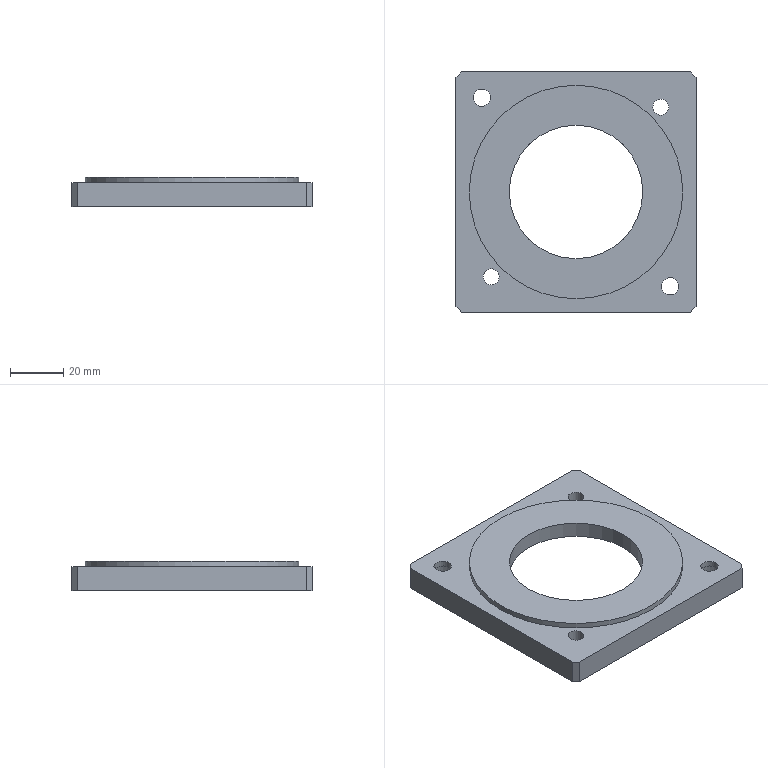NC program | NX | posted with a generic post | part box 90 x 90 x 11 mm
Lines 1 to 1755 of 1862, first 1544 of 1739 lines:
N10 G17 G21 G94 G90
(FLOOR_WALL , TOOL : D50)
N12 T15 M6
N14 G54
N16 G17 G0 G90 X-76.5 Y48.497 S6500 M3
N18 G43 Z30. H15
N20 Z3.
N22 G94 G1 Z0. F1250.
N24 X-73.5
N26 X73.5
N28 Y9.999
N30 X-73.5
N32 Y-28.5
N34 X73.5
N36 X76.5
N38 Z3.
N40 G0 Z30.
N42 M5
(ADAPTIVE_MILLING , TOOL : D10)
N44 T10 M6
N46 G54
N48 G17 G0 G90 X-56.209 Y-0.062 S9500 M3
N50 G43 Z30. H10
N52 Z-8.
N54 G94 G1 Z-11. F1000.
N56 X-55.429 Y-0.341 F3000.
N58 X-54.64 Y-0.597
N60 G3 X-53.562 Y-0.062 R1.017
N62 X-52.789 Y3.126 R8.525
N64 X-52.52 Y12.494 R110.617
N66 G1 X-52.514 Y14.619
N68 X-52.511 Y17.994
N70 X-52.51 Y26.869
N72 X-52.509 Y45.369
N74 Y45.494
N76 X-52.507 Y45.619
N78 G2 X-50.114 Y49.825 R5.686
N80 X-44.574 Y51.965 R12.187
N82 X-36.471 Y52.453 R57.565
N84 G1 X-35.471 Y52.463
N86 X-34.346 Y52.471
N88 X-32.721 Y52.479
N90 X-30.596 Y52.484
N92 X-27.096 Y52.487
N94 X-17.221 Y52.488
N96 X28.779
N98 X29.529 Y52.492
N100 X30.654 Y52.493
N102 X31.529
N104 X32.279 Y52.496
N106 X33.404 Y52.495
N108 G2 X46.028 Y52.466 R533.587
N110 X50.208 Y49.565 R6.086
N112 X52.064 Y43.911 R13.666
N114 X52.471 Y34.426 R81.29
N116 G1 X52.478 Y32.926
N118 X52.483 Y30.801
N120 X52.487 Y27.426
N122 X52.488 Y19.051
N124 X52.489 Y-29.449
N126 X52.495 Y-30.949
N128 X52.494 Y-32.449
N130 X52.496 Y-33.074
N132 Y-34.199
N134 X52.495 Y-34.824
N136 X52.498 Y-35.699
N138 X52.497 Y-36.699
N140 X52.499 Y-37.699
N142 X52.497 Y-38.949
N144 X52.498 Y-39.574
N146 X52.497 Y-40.949
N148 Y-41.449
N150 X52.499 Y-42.449
N152 X52.497 Y-43.574
N154 X52.499 Y-44.324
N156 X52.498 Y-45.324
N158 X52.497 Y-45.574
N160 X52.494 Y-45.699
N162 X52.487 Y-45.824
N164 X52.475 Y-45.949
N166 G2 X49.63 Y-50.163 R6.032
N168 X43.988 Y-52.053 R13.529
N170 X34.878 Y-52.467 R76.098
N172 G1 X33.503 Y-52.475
N174 X31.628 Y-52.481
N176 X28.878 Y-52.485
N178 X23.503 Y-52.487
N180 X-45.497 Y-52.488
N182 X-45.622 Y-52.486
N184 G2 X-49.826 Y-50.086 R5.702
N186 X-51.945 Y-44.67 R12.092
N188 X-52.451 Y-36.568 R56.305
N190 G1 X-52.462 Y-35.568
N192 X-52.47 Y-34.443
N194 X-52.477 Y-33.068
N196 X-52.483 Y-31.068
N198 X-52.486 Y-27.943
N200 X-52.488 Y-21.068
N202 Y-3.818
N204 X-52.487 Y-3.693
N206 X-52.485 Y-3.568
N208 X-52.478 Y-3.318
N210 X-52.473 Y-3.193
N212 G2 X-51.832 Y3.148 R397.339
N214 G3 X-51.526 Y17.267 R210.01
N216 G1 X-51.522 Y20.767
N218 X-51.52 Y28.392
N220 Y42.392
N222 X-51.518 Y42.517
N224 X-51.516 Y42.642
N226 X-51.504 Y42.891
N228 G2 X-47.72 Y48.895 R7.721
N230 X-41.356 Y50.984 R15.76
N232 X-31.249 Y51.454 R84.679
N234 G1 X-29.874 Y51.462
N236 X-28.124 Y51.469
N238 X-25.749 Y51.473
N240 X-21.624 Y51.476
N242 X-7.499 Y51.477
N244 X25.751
N246 G2 X43.125 Y51.466 R849.618
N248 X48.889 Y47.718 R7.741
N250 X50.999 Y41.231 R15.861
N252 X51.45 Y31.748 R82.109
N254 G1 X51.458 Y30.623
N256 X51.466 Y28.998
N258 X51.472 Y26.998
N260 X51.475 Y23.998
N262 X51.477 Y17.748
N264 X51.478 Y-26.502
N266 G2 X51.464 Y-43.126 R752.147
N268 X47.716 Y-48.889 R7.737
N270 X41.229 Y-50.999 R15.895
N272 X31.371 Y-51.452 R84.867
N274 G1 X29.996 Y-51.461
N276 X28.246 Y-51.468
N278 X25.746 Y-51.473
N280 X21.621 Y-51.476
N282 X7.496 Y-51.477
N284 X-42.379
N286 G2 X-48.754 Y-47.906 R7.59
N288 X-50.909 Y-41.829 R14.89
N290 X-51.435 Y-33.102 R65.156
N292 G1 X-51.446 Y-32.102
N294 X-51.456 Y-30.852
N296 X-51.464 Y-29.352
N298 X-51.47 Y-27.352
N300 X-51.475 Y-24.477
N302 X-51.477 Y-18.977
N304 G2 X-51.429 Y-4.228 R621.113
N306 G3 X-50.742 Y5.247 R678.078
N308 X-50.532 Y25.994 R547.933
N310 G2 X-50.492 Y40.743 R710.406
N312 X-50.15 Y42.711 R15.101
N314 X-48.663 Y46.614 R5.592
N316 G1 X-48.617 Y46.666
N318 X-46.666 Y48.617
N320 X-46.614 Y48.663
N322 G2 X-43.034 Y50.145 R5.569
N324 G3 X-33.719 Y50.406 R849.439
N326 G2 X-16.22 Y50.466 R903.691
N328 G1 X22.78
N330 X23.905 Y50.473
N332 X24.905 Y50.474
N334 X25.78 Y50.475
N336 X26.655 Y50.479
N338 X27.405 Y50.481
N340 G2 X40.779 Y50.46 R547.914
N342 X42.624 Y50.15 R18.518
N344 X45.63 Y49.418 R5.935
N346 G1 X46.614 Y48.663
N348 X46.666 Y48.617
N350 X48.617 Y46.666
N352 X48.663 Y46.614
N354 G2 X50.145 Y43.034 R5.569
N356 G3 X50.412 Y33.344 R935.35
N358 G1 X50.426 Y32.095
N360 X50.438 Y30.72
N362 X50.447 Y29.095
N364 X50.456 Y27.095
N366 X50.461 Y24.595
N368 X50.465 Y20.845
N370 X50.467 Y12.72
N372 Y-23.53
N374 X50.473 Y-24.655
N376 X50.474 Y-25.655
N378 X50.475 Y-26.655
N380 X50.481 Y-27.655
N382 G2 X50.459 Y-40.779 R542.291
N384 X50.15 Y-42.62 R17.941
N386 X49.418 Y-45.63 R5.937
N388 G1 X48.663 Y-46.614
N390 X48.617 Y-46.666
N392 X46.666 Y-48.617
N394 X46.614 Y-48.663
N396 G2 X43.034 Y-50.145 R5.569
N398 G3 X33.469 Y-50.409 R920.282
N400 G2 X14.095 Y-50.466 R996.301
N402 G1 X-39.78
N404 X-40.03 Y-50.464
N406 X-40.28 Y-50.458
N408 X-40.405 Y-50.454
N410 X-40.655 Y-50.441
N412 G2 X-42.517 Y-50.15 R16.061
N414 X-45.63 Y-49.418 R5.996
N416 G1 X-46.614 Y-48.663
N418 X-46.666 Y-48.617
N420 X-48.617 Y-46.666
N422 X-48.663 Y-46.614
N424 G2 X-50.145 Y-43.034 R5.569
N426 G3 X-50.402 Y-33.844 R791.933
N428 G1 X-50.417 Y-32.719
N430 X-50.43 Y-31.47
N432 X-50.44 Y-30.22
N434 X-50.449 Y-28.595
N436 X-50.457 Y-26.47
N438 X-50.462 Y-23.97
N440 X-50.465 Y-19.845
N442 G2 X-50.416 Y-5.345 R679.932
N444 G1 X-50.395 Y-4.846
N446 X-50.371 Y-4.346
N448 X-50.344 Y-3.847
N450 X-50.313 Y-3.348
N452 X-50.271 Y-2.724
N454 X-50.191 Y-1.602
N456 X-50.15 Y-1.046
N458 Y42.829
N460 G2 X-49.418 Y45.63 R5.894
N462 G1 X-48.617 Y46.666
N464 X-46.614 Y48.663
N466 G2 X-44.264 Y49.984 R5.901
N468 X-41.965 Y50.15 R11.351
N470 G1 X42.66
N472 G2 X45.63 Y49.418 R5.92
N474 G1 X46.666 Y48.617
N476 X48.663 Y46.614
N478 G2 X49.984 Y44.264 R5.901
N480 X50.15 Y41.84 R11.646
N482 G1 Y-42.66
N484 G2 X49.418 Y-45.63 R5.92
N486 G1 X48.617 Y-46.666
N488 X46.614 Y-48.663
N490 G2 X44.264 Y-49.984 R5.901
N492 X41.84 Y-50.15 R11.646
N494 G1 X-42.535
N496 G2 X-45.63 Y-49.418 R5.985
N498 G1 X-46.666 Y-48.617
N500 X-48.663 Y-46.614
N502 G2 X-49.984 Y-44.264 R5.901
N504 X-50.15 Y-41.84 R11.646
N506 G1 Y-0.965
N508 G3 X-50.998 Y0.032 R1.016
N510 G1 X-52.551 Y0.284
N512 Z-8.
N514 G0 Z30.
N516 X-52.802 Y0.345
N518 Z1.151
N520 G1 Z-1.849 F1000.
N522 X-52.021 Y0.066 F3000.
N524 X-51.233 Y-0.191
N526 G3 X-50.155 Y0.345 R1.017
N528 X-49.394 Y3.409 R8.28
N530 X-49.111 Y13.276 R111.643
N532 G1 X-49.107 Y15.526
N534 X-49.104 Y19.401
N536 X-49.103 Y33.026
N538 Y39.901
N540 X-49.102 Y40.026
N542 X-49.1 Y40.151
N544 G2 X-46.974 Y45.635 R8.713
N546 X-41.836 Y48.307 R10.099
N548 X-34.132 Y49.017 R38.987
N550 X-14.882 Y49.081 R957.171
N552 G1 X39.993
N554 X40.118 Y49.08
N556 X40.242 Y49.078
N558 X40.367 Y49.074
N560 X40.492 Y49.067
N562 X40.617 Y49.058
N564 G2 X45.787 Y46.806 R8.398
N566 X48.354 Y41.609 R10.436
N568 X49.012 Y34.4 R39.109
N570 X49.08 Y21.15 R718.348
N572 G1 X49.081 Y-11.975
N574 Y-40.1
N576 X49.079 Y-40.225
N578 X49.075 Y-40.35
N580 X49.069 Y-40.474
N582 G2 X46.831 Y-45.783 R8.537
N584 X41.753 Y-48.315 R10.23
N586 X34.547 Y-48.991 R37.77
N588 X18.922 Y-49.065 R791.179
N590 G1 X-40.078 Y-49.08
N592 X-40.203 Y-49.079
N594 X-40.328 Y-49.075
N596 X-40.453 Y-49.07
N598 X-40.578 Y-49.062
N600 G2 X-45.769 Y-46.852 R8.524
N602 X-48.352 Y-41.664 R10.293
N604 X-49.009 Y-34.581 R38.201
N606 X-49.08 Y-21.331 R714.275
N608 G1 X-49.081 Y-3.456
N610 X-49.08 Y-3.331
N612 X-49.075 Y-3.081
N614 X-49.072 Y-2.956
N616 X-49.061 Y-2.707
N618 G2 X-48.441 Y3.386 R677.891
N620 G3 X-48.123 Y16.004 R179.253
N622 G1 X-48.118 Y18.629
N624 X-48.115 Y22.879
N626 X-48.113 Y36.129
N628 Y37.004
N630 X-48.109 Y37.504
N632 X-48.104 Y37.754
N634 G2 X-46.562 Y43.071 R9.233
N636 X-41.076 Y46.799 R10.478
N638 X-33.555 Y47.912 R29.339
N640 X-19.557 Y48.068 R385.711
N642 G1 X-12.557 Y48.07
N644 X37.443
N646 X37.568 Y48.069
N648 X37.693 Y48.067
N650 X37.943 Y48.061
N652 X38.068 Y48.056
N654 G2 X43.989 Y45.782 R8.629
N656 X47.123 Y39.907 R11.849
N658 X47.965 Y32.217 R38.476
N660 X48.069 Y17.718 R712.107
N662 G1 X48.07 Y4.593
N664 Y-37.407
N666 X48.068 Y-37.657
N668 X48.066 Y-37.782
N670 X48.059 Y-38.032
N672 X48.054 Y-38.157
N674 G2 X43.105 Y-45.955 R8.584
N676 X36.615 Y-47.671 R18.662
N678 X25.251 Y-48.041 R122.678
N680 G1 X23.251 Y-48.047
N682 X20.376 Y-48.052
N684 X14.626 Y-48.055
N686 X-37.374 Y-48.069
N688 X-37.499 Y-48.068
N690 X-37.624 Y-48.067
N692 G2 X-42.76 Y-46.758 R9.416
N694 X-46.725 Y-41.303 R10.165
N696 X-47.896 Y-33.919 R27.464
N698 X-48.069 Y-17.546 R401.563
N700 X-48.018 Y-3.797 R500.362
N702 G3 X-47.32 Y6.052 R462.364
N704 X-47.126 Y24.55 R515.339
N706 G2 X-47.064 Y36.674 R391.589
N708 X-41.956 Y44.594 R9.378
N710 X-34.907 Y46.603 R19.29
N712 X-24.671 Y47.033 R100.142
N714 G1 X-23.171 Y47.042
N716 X-21.296 Y47.049
N718 X-18.796 Y47.055
N720 X-14.796 Y47.058
N722 X-4.796 Y47.06
N724 X35.204
N726 G2 X40.208 Y46.18 R11.551
N728 X45.158 Y40.773 R10.187
N730 X46.755 Y33.352 R23.648
N732 X47.047 Y21.983 R163.986
N734 G1 X47.053 Y19.733
N736 X47.057 Y16.483
N738 X47.059 Y9.858
N740 X47.06 Y-35.142
N742 X47.058 Y-35.392
N744 X47.053 Y-35.767
N746 G2 X45.021 Y-42.057 R9.669
N748 X38.943 Y-45.803 R12.014
N750 X30.91 Y-46.885 R34.429
N752 X15.412 Y-47.043 R470.302
N754 G1 X6.162 Y-47.047
N756 X-35.088 Y-47.058
N758 X-35.463 Y-47.055
N760 X-35.713 Y-47.053
N762 X-36.088 Y-47.044
N764 X-36.338 Y-47.035
N766 G2 X-44.679 Y-41.785 R9.402
N768 X-46.613 Y-34.842 R19.415
N770 X-47.035 Y-24.481 R102.047
N772 G1 X-47.043 Y-23.106
N774 X-47.05 Y-21.356
N776 X-47.055 Y-18.856
N778 X-47.058 Y-14.731
N780 X-47.059 Y-7.606
N782 X-47.057 Y-7.106
N784 G2 X-46.533 Y2.504 R187.393
N786 G3 X-46.145 Y19.621 R286.661
N788 G2 X-46.073 Y34.745 R701.821
N790 X-40.394 Y43.541 R10.158
N792 X-33.212 Y45.552 R20.494
N794 X-21.853 Y46.023 R108.266
N796 G1 X-20.353 Y46.032
N798 X-18.353 Y46.039
N800 X-15.603 Y46.044
N802 X-11.103 Y46.048
N804 X2.397 Y46.049
N806 X33.147
N808 G2 X38.42 Y45.231 R13.214
N810 X43.892 Y39.654 R10.673
N812 X45.664 Y32.147 R23.348
N814 X46.034 Y19.906 R147.756
N816 G1 X46.041 Y17.781
N818 X46.045 Y14.781
N820 X46.048 Y9.656
N822 X46.049 Y-16.719
N824 Y-33.219
N826 X46.042 Y-33.844
N828 G2 X44.44 Y-39.918 R10.848
N830 X38.305 Y-44.421 R11.796
N832 X30.447 Y-45.783 R29.546
N834 X17.451 Y-46.026 R247.642
N836 G1 X14.201 Y-46.032
N838 X8.201 Y-46.035
N840 X-33.174 Y-46.046
N842 X-33.674 Y-46.044
N844 X-34.049 Y-46.038
N846 X-34.424 Y-46.026
N848 G2 X-43.575 Y-40.307 R10.166
N850 X-45.595 Y-32.871 R20.985
N852 X-46.027 Y-21.384 R118.173
N854 X-45.989 Y-5.76 R614.756
N856 G3 X-45.275 Y9.097 R676.94
N858 X-45.132 Y30.096 R982.975
N860 G2 X-44.787 Y35.199 R25.006
N862 X-38.871 Y42.528 R10.781
N864 X-31.303 Y44.548 R22.208
N866 X-19.317 Y45.014 R121.813
N868 G1 X-17.567 Y45.023
N870 X-15.567 Y45.029
N872 X-12.692 Y45.034
N874 X-7.817 Y45.037
N876 X-2.695 Y45.038
N878 G2 X2.475 Y45.081 R45.644
N880 G1 X3.975 Y45.068
N882 X5.35 Y45.06
N884 X6.724 Y45.055
N886 X8.099 Y45.054
N888 X9.224 Y45.055
N890 X9.849 Y45.053
N892 X11.224 Y45.052
N894 X12.224 Y45.053
N896 X13.224 Y45.05
N898 X14.724 Y45.053
N900 X15.599 Y45.05
N902 X16.474 Y45.051
N904 X17.724 Y45.048
N906 X18.974 Y45.051
N908 G2 X33.099 Y45.001 R617.655
N910 X42.536 Y38.817 R10.77
N912 X44.568 Y31.124 R22.445
N914 X45.008 Y20.138 R115.245
N916 G1 X45.019 Y18.513
N918 X45.026 Y16.888
N920 X45.032 Y14.388
N922 X45.036 Y10.638
N924 X45.038 Y3.138
N926 Y2.835
N928 G2 X45.08 Y-4.633 R105.576
N930 G1 X45.072 Y-6.008
N932 X45.066 Y-7.758
N934 X45.062 Y-10.383
N936 X45.06 Y-15.508
N938 Y-30.258
N940 X45.055 Y-31.008
N942 G2 X44.463 Y-36.202 R17.067
N944 X38.667 Y-42.596 R10.881
N946 X31.081 Y-44.556 R22.797
N948 X19.594 Y-44.997 R122.648
N950 G1 X17.969 Y-45.006
N952 X15.969 Y-45.014
N954 X13.094 Y-45.019
N956 X8.469 Y-45.024
N958 X3.032 Y-45.026
N960 G2 X-4.1 Y-45.075 R86.171
N962 G1 X-5.1 Y-45.068
N964 X-6.6 Y-45.061
N966 X-8.6 Y-45.056
N968 X-11.725 Y-45.054
N970 X-18.975
N972 X-30.225 Y-45.056
N974 G2 X-35.326 Y-44.702 R23.76
N976 X-42.537 Y-38.82 R10.772
N978 X-44.526 Y-31.5 R21.773
N980 X-45.01 Y-20.141 R108.059
N982 X-44.914 Y-4.893 R343.056
N984 G3 X-44.99 Y-3.781 R5.445
N986 G1 X-45.148 Y0.331
N988 X-44.929 Y4.448
N990 X-44.924 Y4.497
N992 G3 X-44.238 Y13.461 R57.287
N994 G1 X-44.223 Y14.336
N996 X-44.208 Y15.461
N998 X-44.195 Y16.711
N1000 X-44.185 Y18.086
N1002 X-44.175 Y19.961
N1004 X-44.167 Y22.211
N1006 X-44.161 Y25.211
N1008 X-44.15 Y26.711
N1010 X-44.148 Y27.461
N1012 X-44.14 Y28.461
N1014 X-44.129 Y29.46
N1016 X-44.12 Y30.085
N1018 X-44.112 Y30.46
N1020 X-44.105 Y30.71
N1022 G2 X-42.336 Y37.263 R12.523
N1024 X-35.889 Y42.173 R12.658
N1026 X-27.81 Y43.703 R29.71
N1028 X-13.816 Y44.018 R215.208
N1030 G1 X-10.941 Y44.023
N1032 X-9.941 Y44.024
N1034 X-9.816 Y44.03
N1036 X-9.784 Y44.033
N1038 X-8.391 Y44.362
N1040 X-8.344 Y44.371
N1042 X-4.287 Y44.945
N1044 X-4.243 Y44.949
N1046 X-0.903 Y45.14
N1048 X-0.879 Y45.141
N1050 X2.475 Y45.081
N1052 G2 X8.351 Y44.371 R57.662
N1054 G3 X16.967 Y44.075 R92.067
N1056 G2 X31.217 Y44.007 R868.307
N1058 X38.572 Y41.301 R11.514
N1060 X42.609 Y34.519 R14.11
N1062 X43.833 Y25.624 R38.889
N1064 X44.032 Y9.769 R450.651
N1066 G1 X44.51 Y7.566
N1068 X44.519 Y7.518
N1070 X45.018 Y3.439
N1072 X45.021 Y3.39
N1074 X45.04 Y2.765
N1076 G3 X46.648 Y2.002 R1.002
N1078 X47.043 Y2.622 Z-1.812 R1.224
N1080 G1 X47.485 Y3.793 Z-1.749
N1082 X48.195 Y5.699
N1084 X48.222 Y5.947
N1086 X48.17 Y9.319
N1088 X48.068 Y12.689
N1090 X47.931 Y14.933
N1092 X47.748 Y17.172
N1094 X46.55 Y29.756
N1096 G3 X44.724 Y37.824 R32.889
N1098 X41.744 Y42.425 R13.191
N1100 G1 X40.117 Y44.036
N1102 G3 X38.414 Y45.179 R7.647
N1104 X35.662 Y46.344 R26.625
N1106 X33.718 Y46.728 R8.766
N1108 X25.617 Y47.203 R154.579
N1110 G1 X10.913 Y47.633
N1112 X10.71 Y47.614
N1114 X10.512 Y47.562
N1116 X8.706 Y46.839
N1118 X8.048 Y46.577 Z-1.784
N1120 X7.395 Y46.302 Z-1.82
N1122 G3 X7.003 Y45.882 Z-1.849 R1.051
N1124 X7.731 Y44.451 R1.003
N1126 G2 X11.646 Y43.595 R39.336
N1128 G3 X18.997 Y43.113 R47.939
N1130 G2 X29.871 Y42.993 R594.457
N1132 X37.151 Y40.386 R12.045
N1134 X41.392 Y33.732 R14.01
N1136 X42.78 Y24.738 R36.574
N1138 X43.024 Y13.532 R352.44
N1140 X44.036 Y9.75 R25.435
N1142 G3 X45.994 Y9.769 R1.
N1144 G1 X46.149 Y11.763 Z-1.749
N1146 X46.286 Y13.647
N1148 X46.289 Y17.395
N1150 X46.272 Y21.144
N1152 G3 X45.392 Y29.816 R56.113
N1154 G1 X44.709 Y33.501
N1156 G3 X42.554 Y38.63 R15.172
N1158 G1 X42.193 Y39.135
N1160 X41.816 Y39.629
N1162 X40.865 Y40.804
N1164 X39.902 Y41.969
N1166 G3 X34.025 Y45.353 R10.912
N1168 X28.477 Y46.122 R33.819
N1170 G1 X14.46 Y46.851
N1172 X14.236 Y46.834
N1174 X14.02 Y46.774
N1176 X12.236 Y46.022
N1178 X11.611 Y45.764 Z-1.783
N1180 X10.995 Y45.485 Z-1.817
N1182 G3 X10.592 Y44.993 Z-1.849 R1.042
N1184 X11.278 Y43.669 R1.004
N1186 G2 X14.682 Y42.721 R87.973
N1188 G3 X21.648 Y42.143 R39.423
N1190 G2 X29.393 Y41.917 R116.86
N1192 X39.404 Y34.824 R12.046
N1194 X41.51 Y26.503 R25.325
N1196 X41.965 Y16.642 R121.15
N1198 G3 X42.387 Y15.548 R20.046
N1200 G1 X43.027 Y13.522
N1202 G3 X44.814 Y13.269 R1.001
N1204 X44.994 Y13.94 Z-1.814 R1.286
N1206 G1 X45.101 Y15.231 Z-1.749
N1208 X45.277 Y17.419
N1210 X45.266 Y21.434
N1212 G3 X44.718 Y26.744 R35.25
N1214 G1 X43.998 Y30.633
N1216 G3 X42.231 Y35.906 R24.086
N1218 X40.361 Y38.908 R17.781
N1220 G1 X39.408 Y40.143
N1222 X38.419 Y41.351
N1224 G3 X37.476 Y42.151 R4.49
N1226 G1 X35.96 Y43.084
N1228 G3 X32.996 Y44.213 R11.072
N1230 X27.468 Y45.126 R43.094
N1232 G1 X17.02 Y46.133
N1234 G3 X16.512 Y46.048 R1.113
N1236 G1 X14.808 Y45.277
N1238 X14.206 Y45.01 Z-1.782
N1240 X13.614 Y44.72 Z-1.815
N1242 G3 X13.217 Y44.182 Z-1.849 R1.039
N1244 X13.838 Y42.951 R1.005
N1246 X17.515 Y41.738 R31.119
N1248 X23.482 Y41.185 R37.684
N1250 G2 X29.457 Y40.72 R39.057
N1252 X38.205 Y33.918 R12.26
N1254 X40.386 Y26.004 R24.116
N1256 X40.887 Y19.15 R105.544
N1258 G1 X40.909 Y19.069
N1260 X42.023 Y16.419
N1262 G3 X43.625 Y16.074 R1.002
N1264 X43.96 Y16.902 Z-1.803 R1.162
N1266 G1 X44.068 Y17.978 Z-1.749
N1268 X44.283 Y20.196
N1270 X43.659 Y24.649
N1272 X43.007 Y29.099
N1274 G3 X41.676 Y33.764 R21.885
N1276 X39.562 Y37.561 R22.014
N1278 X37.525 Y39.892 R16.542
N1280 G1 X36.306 Y41.027
N1282 G3 X34.015 Y42.401 R8.815
N1284 X28.019 Y44.03 R25.085
N1286 G1 X19.609 Y45.207
N1288 G3 X19.052 Y45.124 R1.053
N1290 G1 X17.393 Y44.358
N1292 X16.79 Y44.086 Z-1.782
N1294 X16.198 Y43.791 Z-1.815
N1296 G3 X15.807 Y43.255 Z-1.849 R1.039
N1298 X16.427 Y42.025 R1.005
N1300 G2 X18.653 Y41.109 R52.658
N1302 G3 X23.95 Y40.277 R22.825
N1304 G2 X29.855 Y39.314 R23.93
N1306 X37.337 Y32.37 R12.837
N1308 X39.44 Y24.046 R26.276
N1310 G1 X39.493 Y23.548
N1312 X39.53 Y23.175
N1314 X39.564 Y22.802
N1316 X39.597 Y22.428
N1318 X39.638 Y21.93
N1320 X39.66 Y21.681
N1322 X39.677 Y21.557
N1324 X39.706 Y21.435
N1326 G2 X40.922 Y19.036 R100.794
N1328 G3 X42.5 Y18.669 R1.003
N1330 X42.859 Y19.511 Z-1.802 R1.147
N1332 G1 X42.969 Y20.562 Z-1.749
N1334 X43.092 Y21.672
N1336 X43.191 Y22.784
N1338 X43.172 Y22.934
N1340 X42.263 Y27.424
N1342 G3 X41.071 Y31.404 R32.108
N1344 G1 X40.634 Y32.573
N1346 X40.147 Y33.723
N1348 G3 X38.14 Y36.87 R15.839
N1350 G1 X36.286 Y39.117
N1352 G3 X33.859 Y40.959 R8.899
N1354 X31.33 Y42.013 R18.304
N1356 X28.311 Y42.756 R18.302
N1358 X21.863 Y43.593 R96.615
N1360 G1 X19.662 Y43.37
N1362 X18.248 Y43.213 Z-1.82
N1364 G3 X17.759 Y42.923 Z-1.849 R1.052
N1366 X18.071 Y41.337 R1.003
N1368 X21.171 Y40.013 R22.253
N1370 X26.082 Y39.087 R67.839
N1372 G2 X36.424 Y30.941 R13.505
N1374 X38.29 Y23.958 R26.989
N1376 G3 X38.821 Y23.052 R4.894
N1378 G1 X39.762 Y21.287
N1380 G3 X41.193 Y20.922 R1.004
N1382 X41.648 Y21.711 Z-1.802 R1.046
N1384 G1 X41.798 Y22.756 Z-1.749
N1386 X42.074 Y24.671
N1388 G3 X42.012 Y25.184 R1.112
N1390 G1 X40.701 Y28.473
N1392 X39.371 Y31.755
N1394 G3 X36.83 Y36.41 R30.713
N1396 X34.151 Y39.08 R10.723
N1398 X27.922 Y41.803 R16.802
N1400 G1 X24.008 Y42.638
N1402 X23.849 Y42.654
N1404 X23.688
N1406 X21.681 Y42.429
N1408 X20.979 Y42.353 Z-1.784
N1410 X20.278 Y42.261 Z-1.82
N1412 G3 X19.786 Y41.959 Z-1.849 R1.051
N1414 X20.111 Y40.388 R1.003
N1416 G1 X22.26 Y39.305
N1418 G3 X26.55 Y37.954 R101.071
N1420 G2 X35.627 Y29.267 R14.434
N1422 X36.571 Y26.471 R63.339
N1424 G1 X38.428 Y23.652
N1426 G3 X40.189 Y23.825 R1.002
N1428 X40.215 Y24.563 Z-1.812 R1.222
N1430 G1 X40.002 Y25.793 Z-1.749
N1432 X39.631 Y27.891
N1434 G3 X38.041 Y31.397 R40.926
N1436 G1 X36.871 Y33.606
N1438 G3 X33.662 Y37.372 R14.578
N1440 X27.921 Y40.836 R23.55
N1442 G1 X26.638 Y41.388
N1444 X25.348 Y41.92
N1446 X25.142 Y41.949
N1448 X24.934 Y41.943
N1450 X23.087 Y41.656
N1452 X22.427 Y41.559 Z-1.782
N1454 X21.771 Y41.438 Z-1.816
N1456 G3 X21.252 Y41.042 Z-1.849 R1.04
N1458 X21.582 Y39.625 R1.004
N1460 X26.984 Y36.746 R59.798
N1462 G2 X33.907 Y29.811 R16.165
N1464 G1 X33.94 Y29.775
N1466 X36.506 Y26.565
N1468 X36.535 Y26.526
N1470 X36.604 Y26.421
N1472 G3 X38.272 Y27.831 R-1.1
N1474 G1 X25.154 Y40.058
N1476 G3 X23.85 Y38.303 R-1.1
N1478 G1 X24.484 Y37.933
N1480 X24.525 Y37.907
N1482 X27.871 Y35.52
N1484 X27.909 Y35.489
N1486 X31.021 Y32.805
N1488 X31.056 Y32.771
N1490 X33.907 Y29.811
N1492 G3 X34.923 Y29.55 R1.011
N1494 G1 X36.83 Y30.151 Z-1.749
N1496 X37.4 Y30.315
N1498 G2 X38.407 Y29.811 R1.01
N1500 G1 X42.669 Y22.174
N1502 G2 X44.787 Y17.664 R36.62
N1504 X46.73 Y12.171 R93.567
N1506 X47.591 Y8.113 R26.437
N1508 G1 X48.325 Y2.423
N1510 G2 X47.867 Y1.449 R1.011
N1512 G1 X47.603 Y1.283
N1514 X45.911 Y0.216 Z-1.849
N1516 X45.626 Y0.038
N1518 X45.372 Y-0.182
N1520 G3 X45.143 Y-0.759 R1.044
N1522 G1 X44.886 Y-4.868
N1524 X44.88 Y-4.917
N1526 G3 X44.105 Y-14.37 R49.31
N1528 G1 X44.096 Y-15.245
N1530 X44.087 Y-16.495
N1532 X44.08 Y-18.12
N1534 X44.075 Y-20.37
N1536 X44.072 Y-24.12
N1538 X44.071 Y-27.245
N1540 X44.064 Y-28.37
N1542 X44.051 Y-29.87
N1544 G2 X43.167 Y-35.516 R15.362
N1546 X37.058 Y-41.651 R11.565
N1548 X29.325 Y-43.55 R24.504
N1550 X16.587 Y-43.992 R139.689
N1552 G1 X14.587 Y-44.001
N1554 X11.962 Y-44.007
N1556 X9.962 Y-44.01
N1558 X9.831 Y-44.018
N1560 X7.729 Y-44.482
N1562 X7.681 Y-44.491
N1564 X3.6 Y-45.005
N1566 X3.551 Y-45.009
N1568 X2.926 Y-45.03
N1570 G3 X2.162 Y-46.632 R1.002
N1572 X2.786 Y-47.032 Z-1.811 R1.219
N1574 G1 X3.951 Y-47.472 Z-1.749
N1576 X5.859 Y-48.184
N1578 X6.108 Y-48.212
N1580 X9.48 Y-48.16
N1582 X12.85 Y-48.058
N1584 X15.093 Y-47.921
N1586 X17.333 Y-47.738
N1588 X31.024 Y-46.434
N1590 G3 X38.496 Y-44.366 R21.908
N1592 X41.905 Y-42.276 R26.005
N1594 X44.584 Y-39.355 R11.528
N1596 X46.054 Y-36.439 R11.995
N1598 X46.634 Y-33.995 R21.808
N1600 X47.076 Y-29.872 R27.047
N1602 G1 X47.6 Y-11.063
N1604 X47.581 Y-10.861
N1606 X47.53 Y-10.665
N1608 X46.811 Y-8.861
N1610 X46.273 Y-7.537 Z-1.821
N1612 G3 X45.867 Y-7.148 Z-1.849 R1.054
N1614 X44.418 Y-7.881 R1.003
N1616 G2 X43.612 Y-11.574 R35.137
N1618 G3 X43.127 Y-18.8 R46.489
N1620 G2 X42.998 Y-29.924 R444.466
N1622 X39.763 Y-37.836 R11.815
N1624 X32.713 Y-41.674 R15.103
N1626 X23.303 Y-42.835 R44.331
N1628 X13.68 Y-42.995 R602.017
N1630 X9.793 Y-44.026 R30.581
N1632 G3 X9.795 Y-45.979 R1.
N1634 G1 X10.791 Y-46.067 Z-1.799
N1636 X11.788 Y-46.137 Z-1.749
N1638 X13.69 Y-46.276
N1640 X17.673 Y-46.28
N1642 X21.656 Y-46.264
N1644 G3 X29.244 Y-45.493 R49.125
N1646 G1 X31.904 Y-44.996
N1648 G3 X37.177 Y-43.229 R24.086
N1650 X40.179 Y-41.36 R17.781
N1652 G1 X41.414 Y-40.406
N1654 X42.622 Y-39.418
N1656 G3 X43.415 Y-38.471 R4.292
N1658 X45.008 Y-35.098 R13.902
N1660 X45.779 Y-31.46 R14.802
N1662 X46.439 Y-22.119 R357.528
N1664 G1 X46.87 Y-14.389
N1666 X46.853 Y-14.163
N1668 X46.793 Y-13.945
N1670 X46.042 Y-12.163
N1672 X45.784 Y-11.537 Z-1.783
N1674 X45.505 Y-10.92 Z-1.817
N1676 G3 X45.015 Y-10.517 Z-1.849 R1.042
N1678 X43.688 Y-11.207 R1.004
N1680 G2 X42.738 Y-14.608 R65.783
N1682 G3 X42.169 Y-21.199 R36.801
N1684 G2 X41.957 Y-29.07 R159.041
N1686 X34.883 Y-39.362 R12.072
N1688 X26.817 Y-41.461 R24.79
N1690 X16.707 Y-41.948 R112.671
N1692 G3 X15.711 Y-42.327 R9.518
N1694 G1 X13.449 Y-43.051
N1696 G3 X13.19 Y-44.83 R1.002
N1698 X13.868 Y-45.017 Z-1.813 R1.274
N1700 G1 X15.15 Y-45.123 Z-1.749
N1702 X17.346 Y-45.301
N1704 X21.361 Y-45.29
N1706 G3 X26.67 Y-44.742 R35.25
N1708 G1 X30.56 Y-44.022
N1710 G3 X35.833 Y-42.255 R24.086
N1712 X38.835 Y-40.385 R17.781
N1714 X41.747 Y-38.03 R56.067
N1716 X43.139 Y-36.039 R5.2
N1718 G1 X43.621 Y-34.797
N1720 X44.058 Y-33.538
N1722 G3 X44.791 Y-30.072 R20.141
N1724 X46.152 Y-16.947 R462.958
N1726 G1 X46.14 Y-16.689
N1728 X46.068 Y-16.441
N1730 X45.298 Y-14.734
N1732 X45.031 Y-14.13 Z-1.782
N1734 X44.742 Y-13.537 Z-1.815
N1736 G3 X44.205 Y-13.141 Z-1.849 R1.039
N1738 X42.97 Y-13.765 R1.005
N1740 X41.711 Y-17.688 R29.848
N1742 X41.157 Y-24.659 R47.187
N1744 G2 X40.446 Y-30.6 R24.238
N1746 X33.632 Y-38.326 R12.396
N1748 X25.317 Y-40.455 R25.44
N1750 X19.208 Y-40.862 R125.903
N1752 G1 X19.087 Y-40.894
N1754 X16.441 Y-42.019
N1756 G3 X16.095 Y-43.615 R1.003
N1758 X16.926 Y-43.954 Z-1.803 R1.159
N1760 G1 X17.997 Y-44.062 Z-1.749
N1762 X20.217 Y-44.279
N1764 X24.671 Y-43.655
N1766 X29.121 Y-43.003
N1768 G3 X33.786 Y-41.671 R21.885
N1770 X37.583 Y-39.557 R22.014
N1772 X39.914 Y-37.521 R16.542
N1774 G1 X41.049 Y-36.302
N1776 G3 X42.421 Y-34.01 R8.785
N1778 X44.041 Y-28.012 R25.047
N1780 G1 X45.196 Y-19.658
N1782 G3 X45.114 Y-19.103 R1.054
N1784 G1 X44.349 Y-17.44
N1786 X44.077 Y-16.837 Z-1.782
N1788 X43.783 Y-16.244 Z-1.815
N1790 G3 X43.248 Y-15.852 Z-1.849 R1.039
N1792 X42.014 Y-16.476 R1.005
N1794 G1 X41.093 Y-18.699
N1796 G3 X40.324 Y-23.503 R22.601
N1798 G2 X39.489 Y-29.306 R28.476
N1800 X32.425 Y-37.293 R12.801
N1802 X24.357 Y-39.392 R25.475
N1804 G1 X23.984 Y-39.434
N1806 X23.611 Y-39.474
N1808 X23.238 Y-39.51
N1810 X22.74 Y-39.555
N1812 X22.242 Y-39.597
N1814 X21.868 Y-39.628
N1816 X21.743 Y-39.639
N1818 X21.619 Y-39.653
N1820 X21.497 Y-39.68
N1822 G2 X19.082 Y-40.896 R72.057
N1824 G3 X18.722 Y-42.477 R1.003
N1826 X19.56 Y-42.831 Z-1.802 R1.151
N1828 G1 X20.616 Y-42.943 Z-1.749
N1830 X21.721 Y-43.066
N1832 X22.829 Y-43.165
N1834 X22.979 Y-43.146
N1836 X27.469 Y-42.237
N1838 G3 X32.763 Y-40.499 R28.559
N1840 X35.834 Y-38.736 R20.085
N1842 X38.847 Y-36.513 R48.947
N1844 X41.002 Y-33.817 R8.634
N1846 X42.048 Y-31.285 R18.064
N1848 X42.776 Y-28.263 R18.122
N1850 X43.568 Y-21.909 R95.524
N1852 G1 X43.347 Y-19.709
N1854 X43.191 Y-18.289 Z-1.82
N1856 G3 X42.906 Y-17.803 Z-1.849 R1.054
N1858 X41.313 Y-18.114 R1.003
N1860 X39.944 Y-21.463 R19.33
N1862 X39.035 Y-26.379 R136.49
N1864 G2 X30.883 Y-36.436 R13.514
N1866 X24.02 Y-38.264 R26.612
N1868 G3 X23.207 Y-38.728 R3.685
N1870 G1 X21.337 Y-39.736
N1872 G3 X20.973 Y-41.162 R1.004
N1874 X21.763 Y-41.62 Z-1.802 R1.046
N1876 G1 X22.806 Y-41.771 Z-1.749
N1878 X24.85 Y-42.057
N1880 X25.044 Y-42.036
N1882 X25.234 Y-41.986
N1884 X28.775 Y-40.576
N1886 X32.307 Y-39.143
N1888 G3 X35.83 Y-37.152 R19.074
N1890 X37.762 Y-35.336 R12.25
N1892 G1 X38.569 Y-34.386
N1894 X39.336 Y-33.403
N1896 G3 X41.821 Y-27.749 R15.431
N1898 G1 X42.622 Y-24.055
N1900 X42.639 Y-23.894
N1902 Y-23.732
N1904 X42.416 Y-21.73
N1906 X42.248 Y-20.322 Z-1.82
N1908 G3 X41.95 Y-19.833 Z-1.849 R1.051
N1910 X40.372 Y-20.158 R1.003
N1912 G1 X39.332 Y-22.188
N1914 G3 X38.02 Y-26.36 R76.988
N1916 G2 X29.327 Y-35.589 R14.448
N1918 X26.484 Y-36.553 R63.825
N1920 G1 X23.673 Y-38.421
N1922 G3 X23.839 Y-40.176 R1.002
N1924 X24.585 Y-40.207 Z-1.811 R1.214
N1926 G1 X25.807 Y-39.995 Z-1.749
N1928 X27.911 Y-39.625
N1930 G3 X31.418 Y-38.035 R40.914
N1932 G1 X33.627 Y-36.865
N1934 G3 X37.389 Y-33.652 R14.516
N1936 X40.837 Y-27.908 R23.436
N1938 G1 X41.373 Y-26.652
N1940 X41.89 Y-25.388
N1942 X41.919 Y-25.184
N1944 X41.913 Y-24.978
N1946 X41.628 Y-23.127
N1948 X41.532 Y-22.466 Z-1.782
N1950 X41.412 Y-21.808 Z-1.816
N1952 G3 X41.018 Y-21.29 Z-1.849 R1.041
N1954 X39.596 Y-21.622 R1.004
N1956 X36.781 Y-26.917 R61.773
N1958 G2 X29.912 Y-33.818 R15.635
N1960 G1 X26.715 Y-36.397
N1962 X26.675 Y-36.426
N1964 X26.467 Y-36.564
N1966 G3 X27.88 Y-38.231 R-1.1
N1968 G1 X40.041 Y-25.196
N1970 G3 X38.284 Y-23.896 R-1.1
N1972 G2 X35.611 Y-27.754 R62.326
N1974 G1 X32.937 Y-30.88
N1976 X32.904 Y-30.916
N1978 X29.953 Y-33.782
N1980 X29.916 Y-33.815
N1982 X29.819 Y-33.893
N1984 G3 X29.484 Y-34.941 R1.01
N1986 G1 X30.148 Y-36.828 Z-1.749
N1988 X30.265 Y-37.153
N1990 X30.331 Y-37.492
N1992 G2 X29.819 Y-38.393 R1.011
N1994 G1 X22.182 Y-42.655
N1996 G2 X17.672 Y-44.774 R36.682
N1998 X12.18 Y-46.718 R93.833
N2000 X8.122 Y-47.582 R26.55
N2002 G1 X2.457 Y-48.32
N2004 G2 X1.481 Y-47.861 R1.011
N2006 G1 X1.32 Y-47.605
N2008 X0.256 Y-45.912 Z-1.849
N2010 X0.076 Y-45.624
N2012 X-0.146 Y-45.367
N2014 G3 X-0.725 Y-45.138 R1.044
N2016 G1 X-4.716 Y-44.902
N2018 X-4.764 Y-44.897
N2020 G3 X-14.092 Y-44.102 R49.358
N2022 G1 X-14.967 Y-44.092
N2024 X-16.092 Y-44.083
N2026 X-17.466 Y-44.076
N2028 X-19.216 Y-44.071
N2030 X-21.966 Y-44.068
N2032 X-27.341 Y-44.066
N2034 X-28.841 Y-44.056
N2036 X-29.841 Y-44.048
N2038 X-30.341 Y-44.04
N2040 G2 X-36.625 Y-42.657 R13.371
N2042 X-41.952 Y-36.413 R12.112
N2044 X-43.669 Y-28.249 R27.593
N2046 X-44.013 Y-15.257 R181.714
N2048 G1 X-44.02 Y-12.882
N2050 X-44.022 Y-11.132
N2052 X-44.018 Y-10.382
N2054 X-44.014 Y-10.007
N2056 X-44.016 Y-9.882
N2058 X-44.022 Y-9.815
N2060 X-44.446 Y-7.937
N2062 X-44.454 Y-7.889
N2064 X-44.909 Y-4.418
N2066 G3 X-46.351 Y-3.656 R1.003
N2068 X-46.903 Y-4.365 Z-1.803 R1.158
N2070 G1 X-47.295 Y-5.366 Z-1.749
N2072 X-48.062 Y-7.343
N2074 X-48.091 Y-7.6
N2076 X-48.04 Y-10.972
N2078 X-47.937 Y-14.343
N2080 X-47.8 Y-16.586
N2082 X-47.617 Y-18.826
N2084 X-46.55 Y-30.027
N2086 G3 X-45.473 Y-35.618 R29.893
N2088 X-43.742 Y-39.486 R17.93
N2090 G1 X-42.446 Y-41.616
N2092 G3 X-41.47 Y-42.823 R6.676
N2094 X-39.266 Y-44.555 R28.89
N2096 X-35.61 Y-46.329 R13.534
N2098 X-32.91 Y-46.802 R13.421
N2100 X-27.929 Y-47.125 R70.78
N2102 G1 X-11.159 Y-47.589
N2104 X-10.958 Y-47.57
N2106 X-10.762 Y-47.519
N2108 X-8.962 Y-46.803
N2110 X-7.632 Y-46.264 Z-1.821
N2112 G3 X-7.244 Y-45.863 Z-1.849 R1.055
N2114 X-7.977 Y-44.407 R1.003
N2116 G2 X-11.55 Y-43.614 R34.815
N2118 G3 X-18.15 Y-43.133 R41.679
N2120 G2 X-29.774 Y-43.003 R777.446
N2122 X-36.979 Y-40.53 R12.204
N2124 X-41.402 Y-33.711 R13.9
N2126 X-42.782 Y-24.715 R36.462
N2128 X-43.025 Y-13.537 R362.445
N2130 X-44.04 Y-9.736 R26.749
N2132 G3 X-45.986 Y-9.718 R1.001
N2134 G1 X-46.066 Y-10.521 Z-1.809
N2136 X-46.12 Y-11.326 Z-1.768
N2138 X-46.149 Y-11.711 Z-1.749
N2140 X-46.29 Y-13.633
N2142 X-46.292 Y-17.381
N2144 X-46.276 Y-21.13
N2146 G3 X-45.395 Y-29.802 R56.113
N2148 G1 X-44.713 Y-33.487
N2150 G3 X-42.558 Y-38.616 R15.172
N2152 G1 X-42.196 Y-39.121
N2154 X-41.82 Y-39.615
N2156 X-40.869 Y-40.79
N2158 X-39.905 Y-41.955
N2160 G3 X-37.466 Y-43.982 R10.984
N2162 X-35.137 Y-45.155 R11.466
N2164 X-32.217 Y-45.737 R11.26
N2166 G1 X-14.487 Y-46.846
N2168 X-14.258 Y-46.831
N2170 X-14.036 Y-46.77
N2172 X-12.259 Y-46.021
N2174 X-11.633 Y-45.762 Z-1.783
N2176 X-11.015 Y-45.482 Z-1.817
N2178 G3 X-10.613 Y-44.994 Z-1.849 R1.042
N2180 X-11.305 Y-43.664 R1.004
N2182 G2 X-14.464 Y-42.765 R43.352
N2184 G3 X-20.802 Y-42.173 R33.863
N2186 G2 X-29.048 Y-41.957 R183.495
N2188 X-39.417 Y-34.804 R12.091
N2190 X-41.496 Y-26.605 R24.961
N2192 X-41.973 Y-16.62 R124.489
N2194 X-43.039 Y-13.494 R57.487
N2196 G3 X-44.81 Y-13.23 R1.002
N2198 X-45.003 Y-13.916 Z-1.813 R1.25
N2200 G1 X-45.109 Y-15.188 Z-1.749
N2202 X-45.289 Y-17.391
N2204 X-45.277 Y-21.407
N2206 G3 X-44.73 Y-26.716 R35.25
N2208 G1 X-44.009 Y-30.605
N2210 G3 X-42.242 Y-35.878 R24.086
N2212 X-40.373 Y-38.88 R17.781
N2214 G1 X-39.419 Y-40.116
N2216 X-38.431 Y-41.323
N2218 G3 X-37.488 Y-42.124 R4.493
N2220 G1 X-35.47 Y-43.371
N2222 G3 X-31.212 Y-44.666 R11.139
N2224 G1 X-17.044 Y-46.114
N2226 G3 X-16.531 Y-46.03 R1.066
N2228 G1 X-14.827 Y-45.261
N2230 X-14.224 Y-44.994 Z-1.782
N2232 X-13.631 Y-44.705 Z-1.815
N2234 G3 X-13.235 Y-44.168 Z-1.849 R1.039
N2236 X-13.862 Y-42.932 R1.005
N2238 X-17.668 Y-41.714 R31.435
N2240 X-24.888 Y-41.144 R48.271
N2242 G2 X-30.82 Y-40.381 R22.481
N2244 X-38.276 Y-33.781 R12.369
N2246 X-40.375 Y-26.099 R24.241
N2248 X-40.888 Y-19.121 R102.067
N2250 G1 X-40.912 Y-19.033
N2252 X-42.047 Y-16.391
N2254 G3 X-43.637 Y-16.045 R1.003
N2256 X-43.98 Y-16.878 Z-1.803 R1.156
N2258 G1 X-44.088 Y-17.945 Z-1.749
N2260 X-44.306 Y-20.167
N2262 X-43.682 Y-24.621
N2264 X-43.03 Y-29.071
N2266 G3 X-41.699 Y-33.736 R21.885
N2268 X-39.585 Y-37.533 R22.014
N2270 X-36.286 Y-40.984 R18.266
N2272 X-33.336 Y-42.634 R11.96
N2274 X-29.574 Y-43.712 R20.945
N2276 G1 X-28.194 Y-43.967
N2278 X-26.808 Y-44.189
N2280 X-19.641 Y-45.208
N2282 G3 X-19.082 Y-45.126 R1.053
N2284 G1 X-17.42 Y-44.362
N2286 X-16.817 Y-44.09 Z-1.782
N2288 X-16.223 Y-43.795 Z-1.815
N2290 G3 X-15.831 Y-43.261 Z-1.849 R1.039
N2292 X-16.459 Y-42.026 R1.005
N2294 X-18.802 Y-41.058 R112.978
N2296 X-23.983 Y-40.28 R24.671
N2298 G2 X-29.767 Y-39.346 R23.86
N2300 X-37.404 Y-32.232 R12.842
N2302 X-39.462 Y-23.895 R26.956
N2304 G3 X-39.716 Y-21.41 R153.498
N2306 G2 X-40.93 Y-18.991 R29.86
N2308 G3 X-42.511 Y-18.635 R1.003
N2310 X-42.864 Y-19.472 Z-1.802 R1.152
N2312 G1 X-42.976 Y-20.531 Z-1.749
N2314 X-43.1 Y-21.633
N2316 X-43.198 Y-22.737
N2318 X-43.18 Y-22.888
N2320 X-42.271 Y-27.378
N2322 G3 X-40.384 Y-33.095 R33.121
N2324 X-38.688 Y-36.063 R20.009
N2326 X-36.27 Y-39.155 R31.709
N2328 X-33.888 Y-40.926 R9.051
N2330 X-31.944 Y-41.764 R15.645
N2332 X-27.51 Y-42.974 R25.846
N2334 X-23.845 Y-43.455 R27.418
N2336 G1 X-21.995 Y-43.567
N2338 X-21.835 Y-43.564
N2340 X-19.7 Y-43.351
N2342 X-18.274 Y-43.198 Z-1.821
N2344 G3 X-17.791 Y-42.918 Z-1.849 R1.055
N2346 X-18.098 Y-41.317 R1.003
N2348 X-21.446 Y-39.943 R20.658
N2350 X-26.362 Y-39.035 R131.453
N2352 G2 X-36.438 Y-30.915 R13.453
N2354 X-38.303 Y-23.932 R27.756
N2356 G1 X-38.347 Y-23.815
N2358 X-38.389 Y-23.73
N2360 X-38.634 Y-23.364
N2362 X-38.659 Y-23.322
N2364 X-39.792 Y-21.235
N2366 G3 X-41.214 Y-20.872 R1.004
N2368 X-41.675 Y-21.663 Z-1.802 R1.045
N2370 G1 X-41.826 Y-22.704 Z-1.749
N2372 X-42.114 Y-24.747
N2374 X-42.093 Y-24.942
N2376 X-42.042 Y-25.132
N2378 X-40.753 Y-28.366
N2380 X-39.446 Y-31.593
N2382 G3 X-36.258 Y-36.802 R23.417
N2384 X-31.353 Y-40.544 R14.738
N2386 X-28.784 Y-41.641 R21.132
N2388 X-26.344 Y-42.235 R15.947
N2390 G1 X-24.026 Y-42.593
N2392 X-21.826 Y-42.369
N2394 X-21.124 Y-42.297 Z-1.784
N2396 X-20.424 Y-42.21 Z-1.82
N2398 G3 X-19.929 Y-41.908 Z-1.849 R1.05
N2400 X-20.259 Y-40.332 R1.003
N2402 X-22.292 Y-39.289 R56.028
N2404 X-26.822 Y-37.864 R182.6
N2406 G2 X-35.596 Y-29.357 R14.369
N2408 X-36.602 Y-26.401 R68.094
N2410 G1 X-38.409 Y-23.7
N2412 G3 X-40.159 Y-23.862 R1.002
N2414 X-40.193 Y-24.613 Z-1.811 R1.208
N2416 G1 X-39.983 Y-25.829 Z-1.749
N2418 X-39.612 Y-27.938
N2420 G3 X-38.022 Y-31.445 R40.905
N2422 G1 X-36.852 Y-33.654
N2424 G3 X-33.639 Y-37.416 R14.502
N2426 X-27.894 Y-40.86 R23.409
N2428 G1 X-26.585 Y-41.417
N2430 X-25.268 Y-41.956
N2432 X-25.064 Y-41.984
N2434 X-24.859 Y-41.978
N2436 X-23.006 Y-41.695
N2438 X-22.344 Y-41.599 Z-1.782
N2440 X-21.686 Y-41.479 Z-1.816
N2442 G3 X-21.168 Y-41.087 Z-1.849 R1.041
N2444 X-21.501 Y-39.661 R1.004
N2446 X-26.909 Y-36.793 R61.927
N2448 G2 X-33.88 Y-29.826 R15.553
N2450 X-36.625 Y-26.367 R57.102
N2452 G3 X-38.292 Y-27.781 R-1.1
N2454 G1 X-25.296 Y-39.989
N2456 G3 X-23.996 Y-38.232 R-1.1
N2458 G1 X-24.203 Y-38.114
N2460 X-24.244 Y-38.087
N2462 X-27.61 Y-35.723
N2464 X-27.649 Y-35.693
N2466 X-30.782 Y-33.028
N2468 X-30.818 Y-32.995
N2470 X-33.693 Y-30.053
N2472 X-33.726 Y-30.016
N2474 X-33.883 Y-29.822
N2476 G3 X-34.935 Y-29.491 R1.01
N2478 G1 X-36.823 Y-30.153 Z-1.749
N2480 X-37.146 Y-30.268
N2482 X-37.483 Y-30.334
N2484 G2 X-38.383 Y-29.822 R1.011
N2486 G1 X-40.764 Y-25.572
N2488 X-43.123 Y-21.309
N2490 G2 X-46.297 Y-12.933 R38.35
N2492 X-47.76 Y-5.423 R54.936
N2494 X-48.514 Y4.349 R162.77
N2496 X-47.677 Y5.392 R1.005
N2498 G1 X-47.336 Y5.448
N2500 X-45.362 Y5.774 Z-1.849
N2502 G3 X-44.617 Y6.599 R1.01
N2504 G2 X-43.722 Y11.151 R35.829
N2506 G3 X-43.23 Y18.502 R49.424
N2508 G2 X-43.072 Y29.875 R522.568
N2510 X-40.368 Y37.246 R12.072
N2512 X-33.553 Y41.463 R14.189
N2514 X-24.424 Y42.798 R37.775
N2516 X-13.677 Y43.007 R319.101
N2518 X-9.7 Y44.053 R37.855
N2520 G3 X-9.641 Y45.983 R1.001
N2522 G1 X-10.042 Y46.042 Z-1.829
N2524 X-10.447 Y46.068 Z-1.808
N2526 X-11.632 Y46.157 Z-1.749
N2528 X-13.597 Y46.303
N2530 X-17.345 Y46.305
N2532 X-21.093 Y46.289
N2534 G3 X-29.766 Y45.408 R56.113
N2536 G1 X-33.451 Y44.726
N2538 G3 X-39.619 Y41.89 R16.153
N2540 X-42.406 Y39.59 R27.79
N2542 X-43.627 Y38.03 R8.789
N2544 X-45.241 Y34.591 R13.653
N2546 X-45.954 Y30.396 R20.238
N2548 G1 X-46.977 Y13.965
N2550 X-46.961 Y13.737
N2552 X-46.901 Y13.516
N2554 X-46.153 Y11.736
N2556 X-45.894 Y11.108 Z-1.783
N2558 X-45.615 Y10.488 Z-1.817
N2560 G3 X-45.131 Y10.086 Z-1.849 R1.043
N2562 X-43.795 Y10.783 R1.004
N2564 G2 X-42.866 Y14.174 R45.207
N2566 G3 X-42.271 Y20.637 R35.622
N2568 G2 X-42.035 Y29.007 R195.029
N2570 X-35.017 Y39.339 R12.07
N2572 X-26.959 Y41.463 R24.298
N2574 X-16.726 Y41.961 R113.007
N2576 G1 X-16.603 Y41.986
N2578 X-16.52 Y42.009
N2580 X-16.349 Y42.085
N2582 X-16.304 Y42.102
N2584 X-13.46 Y43.058
N2586 G3 X-13.183 Y44.809 R1.002
N2588 X-13.887 Y45.018 Z-1.812 R1.226
N2590 G1 X-15.136 Y45.124 Z-1.749
N2592 X-17.357 Y45.308
N2594 X-21.373 Y45.296
N2596 G3 X-26.682 Y44.749 R35.25
N2598 G1 X-30.571 Y44.028
N2600 G3 X-36.265 Y42.102 R26.964
N2602 X-38.885 Y40.452 R16.458
N2604 X-41.191 Y38.545 R23.751
N2606 X-42.76 Y36.463 R10.512
N2608 X-44.444 Y32.35 R13.546
N2610 X-44.947 Y29.408 R22.922
N2612 G1 X-46.248 Y16.633
N2614 G3 X-46.165 Y16.121 R1.067
N2616 G1 X-45.397 Y14.413
N2618 X-45.131 Y13.809 Z-1.782
N2620 X-44.842 Y13.215 Z-1.815
N2622 G3 X-44.307 Y12.818 Z-1.849 R1.039
N2624 X-43.066 Y13.451 R1.005
N2626 X-41.823 Y17.381 R35.488
N2628 X-41.237 Y24.599 R47.808
N2630 G2 X-40.571 Y30.423 R25.599
N2632 X-33.77 Y38.307 R12.368
N2634 X-25.71 Y40.429 R24.902
N2636 X-19.103 Y40.885 R117.387
N2638 G1 X-18.998 Y40.915
N2640 X-16.482 Y42.026
N2642 G3 X-16.135 Y43.601 R1.003
N2644 X-16.975 Y43.955 Z-1.802 R1.149
N2646 G1 X-18.03 Y44.064 Z-1.749
N2648 X-20.258 Y44.286
N2650 X-24.712 Y43.662
N2652 X-29.162 Y43.01
N2654 G3 X-33.828 Y41.678 R21.885
N2656 X-37.624 Y39.564 R22.014
N2658 X-39.955 Y37.527 R16.542
N2660 G1 X-41.09 Y36.308
N2662 G3 X-42.465 Y34.018 R8.825
N2664 X-44.094 Y28.022 R24.949
N2666 G1 X-45.279 Y19.472
N2668 G3 X-45.198 Y18.919 R1.055
N2670 G1 X-44.435 Y17.25
N2672 X-44.164 Y16.645 Z-1.782
N2674 X-43.871 Y16.051 Z-1.815
N2676 G3 X-43.339 Y15.658 Z-1.849 R1.04
N2678 X-42.097 Y16.29 R1.005
N2680 X-41.039 Y18.978 R24.721
N2682 X-40.321 Y24.424 R31.89
N2684 G2 X-39.185 Y30.418 R20.563
N2686 X-32.24 Y37.429 R12.998
N2688 X-24.02 Y39.448 R26.782
N2690 G3 X-21.411 Y39.717 R44.318
N2692 G2 X-18.951 Y40.935 R23.89
N2694 G3 X-18.596 Y42.5 R1.003
N2696 X-19.439 Y42.865 Z-1.802 R1.145
N2698 G1 X-20.485 Y42.978 Z-1.749
N2700 X-22.545 Y43.199
N2702 X-22.848 Y43.185
N2704 X-27.339 Y42.276
N2706 G3 X-33.056 Y40.389 R33.121
N2708 X-36.025 Y38.694 R20.237
N2710 X-38.683 Y36.678 R30.291
N2712 X-42.25 Y30.877 R12.096
N2714 X-43.034 Y27.223 R33.617
N2716 X-43.646 Y21.81 R47.305
N2718 G1 X-43.644 Y21.641
N2720 X-43.433 Y19.516
N2722 X-43.281 Y18.084 Z-1.821
N2724 G3 X-43.007 Y17.604 Z-1.849 R1.056
N2726 X-41.396 Y17.913 R1.002
N2728 X-40.006 Y21.389 R21.265
N2730 X-39.064 Y26.552 R208.912
N2732 G2 X-30.915 Y36.463 R13.456
N2734 X-24.048 Y38.278 R26.721
N2736 G1 X-23.928 Y38.314
N2738 X-23.812 Y38.36
N2740 X-23.789 Y38.372
N2742 X-23.758 Y38.393
N2744 X-23.716 Y38.418
N2746 X-21.204 Y39.816
N2748 G3 X-20.846 Y41.226 R1.004
N2750 X-21.639 Y41.693 Z-1.801 R1.045
N2752 G1 X-22.674 Y41.845 Z-1.749
N2754 X-24.715 Y42.137
N2756 X-24.911 Y42.117
N2758 X-25.101 Y42.066
N2760 X-28.128 Y40.861
N2762 X-31.146 Y39.632
N2764 G3 X-35.778 Y37.02 R27.112
N2766 G1 X-37.64 Y35.696
N2768 G3 X-39.653 Y33.408 R8.805
N2770 G1 X-40.025 Y32.761
N2772 X-40.36 Y32.094
N2774 X-40.923 Y30.856
N2776 X-41.44 Y29.597
N2778 G3 X-42.295 Y26.329 R18.305
N2780 G1 X-42.689 Y23.846
N2782 X-42.465 Y21.629
N2784 X-42.395 Y20.932 Z-1.784
N2786 X-42.308 Y20.237 Z-1.819
N2788 G3 X-41.998 Y19.736 Z-1.849 R1.048
N2790 X-40.427 Y20.081 R1.003
N2792 X-39.214 Y22.563 R19.069
N2794 G2 X-37.819 Y27.102 R164.209
N2796 X-29.367 Y35.61 R14.337
N2798 X-26.34 Y36.628 R68.344
N2800 G1 X-23.76 Y38.391
N2802 G3 X-23.908 Y40.125 R1.002
N2804 X-24.678 Y40.171 Z-1.81 R1.191
N2806 G1 X-25.874 Y39.966 Z-1.749
N2808 X-27.998 Y39.595
N2810 G3 X-33.239 Y37.083 R44.805
N2812 X-38.245 Y32.844 R18.433
N2814 X-40.188 Y29.552 R13.999
N2816 G1 X-41.953 Y25.311
N2818 G3 X-42.018 Y24.778 R1.06
N2820 G1 X-41.739 Y22.921
N2822 X-41.643 Y22.257 Z-1.783
N2824 X-41.526 Y21.596 Z-1.816
N2826 G3 X-41.139 Y21.079 Z-1.849 R1.041
N2828 X-39.703 Y21.414 R1.004
N2830 X-36.887 Y26.816 R64.221
N2832 G2 X-29.68 Y33.982 R15.597
N2834 X-26.313 Y36.647 R36.592
N2836 G3 X-27.734 Y38.309 R-1.1
N2838 G1 X-40.042 Y25.23
N2840 G3 X-38.308 Y23.893 R-1.1
N2842 G1 X-38.283 Y23.935
N2844 X-35.957 Y27.304
N2846 X-35.927 Y27.343
N2848 X-33.302 Y30.486
N2850 X-33.27 Y30.521
N2852 X-30.368 Y33.41
N2854 X-30.332 Y33.443
N2856 X-29.658 Y34.001
N2858 G3 X-29.444 Y35.312 R1.015
N2860 G1 X-30.309 Y36.705
N2862 Z1.151
N2864 G0 Z30.
N2866 X-2.97 Y-3.285
N2868 Z3.
N2870 G3 X-2.97 Y-3.285 Z2.506 I3.019 J3.337 F1000.
N2872 X-2.97 Y-3.285 Z2.013 I3.019 J3.337
N2874 X-2.97 Y-3.285 Z1.519 I3.019 J3.337
N2876 X-2.97 Y-3.285 Z1.026 I3.019 J3.337
N2878 X-2.97 Y-3.285 Z0.532 I3.019 J3.337
N2880 X-2.97 Y-3.285 Z0.039 I3.019 J3.337
N2882 X-2.97 Y-3.285 Z-0.455 I3.019 J3.337
N2884 X-2.97 Y-3.285 Z-0.948 I3.019 J3.337
N2886 X-2.97 Y-3.285 Z-1.442 I3.019 J3.337
N2888 X-2.97 Y-3.285 Z-1.935 I3.019 J3.337
N2890 X-2.97 Y-3.285 Z-2.429 I3.019 J3.337
N2892 X-2.97 Y-3.285 Z-2.922 I3.019 J3.337
N2894 X-2.97 Y-3.285 Z-3.416 I3.019 J3.337
N2896 X-2.97 Y-3.285 Z-3.909 I3.019 J3.337
N2898 X-2.97 Y-3.285 Z-4.403 I3.019 J3.337
N2900 X-2.97 Y-3.285 Z-4.896 I3.019 J3.337
N2902 X-2.97 Y-3.285 Z-5.39 I3.019 J3.337
N2904 X-2.97 Y-3.285 Z-5.884 I3.019 J3.337
N2906 X-2.97 Y-3.285 Z-6.377 I3.019 J3.337
N2908 X-2.97 Y-3.285 Z-6.871 I3.019 J3.337
N2910 X-2.97 Y-3.285 Z-7.364 I3.019 J3.337
N2912 X-2.97 Y-3.285 Z-7.858 I3.019 J3.337
N2914 X-2.97 Y-3.285 Z-8.351 I3.019 J3.337
N2916 X-2.97 Y-3.285 Z-8.845 I3.019 J3.337
N2918 X-2.97 Y-3.285 Z-9.338 I3.019 J3.337
N2920 X-2.97 Y-3.285 Z-9.832 I3.019 J3.337
N2922 X-2.97 Y-3.285 Z-10.325 I3.019 J3.337
N2924 X-2.97 Y-3.285 Z-10.819 I3.019 J3.337
N2926 X4.55 Y0.052 Z-11. R4.5
N2928 X3.728 Y-2.554 R-4.501 F3000.
N2930 X-1.248 Y4.847 R4.675
N2932 X3.854 Y-3.19 R-4.976
N2934 X-1.917 Y5.144 R5.193
N2936 X3.734 Y-4.023 R-5.473
N2938 X-2.047 Y5.653 R5.716
N2940 X3.859 Y-4.614 R-5.998
N2942 X-2.899 Y5.866 R6.26
N2944 X3.721 Y-5.386 R-6.538
N2946 X-2.51 Y6.651 R6.811
N2948 X3.6 Y-6.125 R-7.1
N2950 X6.435 Y3.933 R7.39
N2952 X-3.581 Y6.792 R7.39
N2954 X3.872 Y-6.644 R-7.682
N2956 X-2.595 Y7.864 R7.973
N2958 X3.52 Y-7.494 R-8.276
N2960 X-2.395 Y8.566 R8.579
N2962 X4.008 Y-7.948 R-8.891
N2964 X-2.312 Y9.235 R9.198
N2966 X3.465 Y-8.87 R-9.517
N2968 X-1.944 Y9.971 R9.832
N2970 X1.254 Y-10.064 R10.152
N2972 X-1.736 Y10.676 R-10.481
N2974 X-10.621 Y-1.772 R10.814
N2976 X1.819 Y-10.658 R10.814
N2978 X-1.262 Y11.418 R11.148
N2980 X0.748 Y-11.451 R11.482
N2982 X-0.027 Y12.166 R11.819
N2984 X-0.618 Y-12.137 R12.16
N2986 X1.991 Y12.694 R12.5
N2988 X-3.73 Y-12.279 R12.84
N2990 X6.613 Y11.788 R13.181
N2992 X-8.241 Y-10.728 R13.518
N2994 X12.235 Y7.03 R13.845
N2996 X-13.278 Y5.228 R14.119
N2998 X6.312 Y-12.911 R14.364
N3000 X-2.724 Y14.769 R14.682
N3002 X0.589 Y-15.016 R15.026
N3004 X5.567 Y14.69 R15.369
N3006 X-9.061 Y-12.843 R15.708
N3008 X13.364 Y9.383 R16.044
N3010 X-15.901 Y4.332 R16.337
N3012 X9.934 Y-13.349 R16.61
N3014 X-5.212 Y16.446 R16.926
N3016 X-0.65 Y-17.251 R17.266
N3018 X10.356 Y14.624 R17.604
N3020 X-17.574 Y-3.803 R17.917
N3022 X17.709 Y-4.792 R18.206
N3024 X-14.466 Y11.964 R18.522
N3026 X1.13 Y-18.782 R18.836
N3028 X8.725 Y17.419 R19.153
N3030 X-18.822 Y-5.177 R19.468
N3032 X12.923 Y-14.9 R19.717
N3034 X17.832 Y-8.701 R19.553
N3036 X19.532 Y-3.511 R22.624
N3038 G1 X19.824 Y-0.913
N3040 X19.831 Y-0.794
N3042 X19.759 Y1.848
N3044 X19.744 Y1.995
N3046 X19.311 Y4.573
N3048 X19.276 Y4.717
N3050 X18.489 Y7.209
N3052 X18.435 Y7.347
N3054 X17.309 Y9.706
N3056 X17.237 Y9.835
N3058 X15.794 Y12.015
N3060 X15.704 Y12.133
N3062 X13.973 Y14.091
N3064 X13.868 Y14.195
N3066 X11.882 Y15.895
N3068 X11.763 Y15.983
N3070 X9.56 Y17.39
N3072 X9.431 Y17.461
N3074 X7.054 Y18.549
N3076 X6.915 Y18.601
N3078 G3 X2.143 Y19.731 R23.724
N3080 X-5.145 Y19.167 R21.438
N3082 X-10.011 Y17.136 R22.817
N3084 X-14.17 Y13.895 R22.817
N3086 X-17.328 Y9.673 R22.817
N3088 X-19.264 Y4.768 R22.817
N3090 X-19.84 Y-0.473 R22.817
N3092 X-19.015 Y-5.681 R22.817